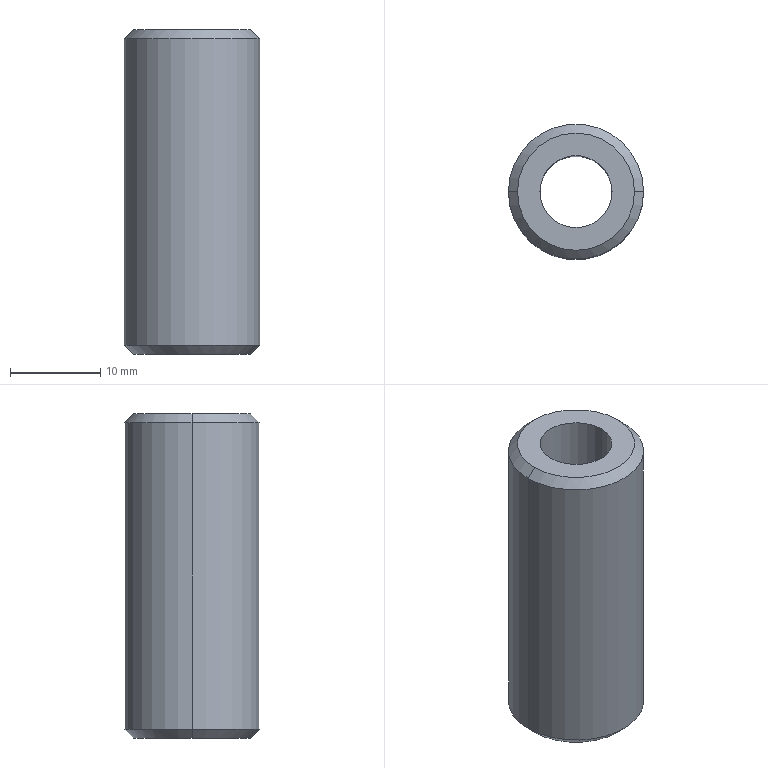Part | SolidWorks | features Chamfer 1, Extrusion 1, ICE 1 | 1 solid | 10 faces | box 15 x 15 x 36 mm | volume 4507 mm3 | cylinder 4 | cone 4 | plane 2 | commonest cylinder face diameters 8 x2 15 x2
STEP:
#1=CARTESIAN_POINT('',(-4.,0.,0.));
#2=VERTEX_POINT('',#1);
#3=CARTESIAN_POINT('',(4.,0.,0.));
#4=VERTEX_POINT('',#3);
#5=CARTESIAN_POINT('',(0.,0.,0.));
#6=DIRECTION('',(0.,0.,1.));
#7=DIRECTION('',(1.,0.,0.));
#8=AXIS2_PLACEMENT_3D('',#5,#6,#7);
#9=CIRCLE('',#8,4.);
#10=EDGE_CURVE('',#2,#4,#9,.T.);
#11=ORIENTED_EDGE('',*,*,#10,.F.);
#12=CARTESIAN_POINT('',(-4.,0.,36.));
#13=VERTEX_POINT('',#12);
#14=CARTESIAN_POINT('',(-4.,0.,0.));
#15=DIRECTION('',(0.,0.,1.));
#16=VECTOR('',#15,1000.);
#17=LINE('',#14,#16);
#18=EDGE_CURVE('',#2,#13,#17,.T.);
#19=ORIENTED_EDGE('',*,*,#18,.T.);
#20=CARTESIAN_POINT('',(4.,0.,36.));
#21=VERTEX_POINT('',#20);
#22=CARTESIAN_POINT('',(0.,0.,36.));
#23=DIRECTION('',(0.,0.,1.));
#24=DIRECTION('',(1.,0.,0.));
#25=AXIS2_PLACEMENT_3D('',#22,#23,#24);
#26=CIRCLE('',#25,4.);
#27=EDGE_CURVE('',#13,#21,#26,.T.);
#28=ORIENTED_EDGE('',*,*,#27,.T.);
#29=CARTESIAN_POINT('',(4.,0.,0.));
#30=DIRECTION('',(0.,0.,1.));
#31=VECTOR('',#30,1000.);
#32=LINE('',#29,#31);
#33=EDGE_CURVE('',#4,#21,#32,.T.);
#34=ORIENTED_EDGE('',*,*,#33,.F.);
#35=EDGE_LOOP('',(#11,#19,#28,#34));
#36=FACE_OUTER_BOUND('',#35,.T.);
#37=CARTESIAN_POINT('',(0.,0.,0.));
#38=DIRECTION('',(0.,0.,1.));
#39=DIRECTION('',(1.,0.,0.));
#40=AXIS2_PLACEMENT_3D('',#37,#38,#39);
#41=CYLINDRICAL_SURFACE('',#40,4.);
#42=ADVANCED_FACE('',(#36),#41,.F.);
#43=CARTESIAN_POINT('',(6.5,0.,36.));
#44=VERTEX_POINT('',#43);
#45=CARTESIAN_POINT('',(-6.5,0.,36.));
#46=VERTEX_POINT('',#45);
#47=CARTESIAN_POINT('',(0.,0.,36.));
#48=DIRECTION('',(0.,0.,1.));
#49=DIRECTION('',(1.,0.,0.));
#50=AXIS2_PLACEMENT_3D('',#47,#48,#49);
#51=CIRCLE('',#50,6.5);
#52=EDGE_CURVE('',#44,#46,#51,.T.);
#53=ORIENTED_EDGE('',*,*,#52,.F.);
#54=CARTESIAN_POINT('',(7.5,0.,35.));
#55=VERTEX_POINT('',#54);
#56=CARTESIAN_POINT('',(6.5,0.,36.));
#57=DIRECTION('',(0.7071,0.,-0.7071));
#58=VECTOR('',#57,1000.);
#59=LINE('',#56,#58);
#60=EDGE_CURVE('',#44,#55,#59,.T.);
#61=ORIENTED_EDGE('',*,*,#60,.T.);
#62=CARTESIAN_POINT('',(-7.5,0.,35.));
#63=VERTEX_POINT('',#62);
#64=CARTESIAN_POINT('',(0.,0.,35.));
#65=DIRECTION('',(0.,0.,-1.));
#66=DIRECTION('',(1.,0.,0.));
#67=AXIS2_PLACEMENT_3D('',#64,#65,#66);
#68=CIRCLE('',#67,7.5);
#69=EDGE_CURVE('',#63,#55,#68,.T.);
#70=ORIENTED_EDGE('',*,*,#69,.F.);
#71=CARTESIAN_POINT('',(-6.5,0.,36.));
#72=DIRECTION('',(-0.7071,0.,-0.7071));
#73=VECTOR('',#72,1000.);
#74=LINE('',#71,#73);
#75=EDGE_CURVE('',#46,#63,#74,.T.);
#76=ORIENTED_EDGE('',*,*,#75,.F.);
#77=EDGE_LOOP('',(#53,#61,#70,#76));
#78=FACE_OUTER_BOUND('',#77,.T.);
#79=CARTESIAN_POINT('',(0.,0.,36.));
#80=DIRECTION('',(0.,0.,-1.));
#81=DIRECTION('',(-1.,0.,0.));
#82=AXIS2_PLACEMENT_3D('',#79,#80,#81);
#83=CONICAL_SURFACE('',#82,6.5,0.7854);
#84=ADVANCED_FACE('',(#78),#83,.T.);
#85=CARTESIAN_POINT('',(-6.5,0.,0.));
#86=VERTEX_POINT('',#85);
#87=CARTESIAN_POINT('',(6.5,0.,0.));
#88=VERTEX_POINT('',#87);
#89=CARTESIAN_POINT('',(0.,0.,0.));
#90=DIRECTION('',(0.,0.,-1.));
#91=DIRECTION('',(1.,0.,0.));
#92=AXIS2_PLACEMENT_3D('',#89,#90,#91);
#93=CIRCLE('',#92,6.5);
#94=EDGE_CURVE('',#86,#88,#93,.T.);
#95=ORIENTED_EDGE('',*,*,#94,.F.);
#96=CARTESIAN_POINT('',(-7.5,0.,1.));
#97=VERTEX_POINT('',#96);
#98=CARTESIAN_POINT('',(-7.5,0.,1.));
#99=DIRECTION('',(-0.7071,0.,0.7071));
#100=VECTOR('',#99,1000.);
#101=LINE('',#98,#100);
#102=EDGE_CURVE('',#86,#97,#101,.T.);
#103=ORIENTED_EDGE('',*,*,#102,.T.);
#104=CARTESIAN_POINT('',(7.5,0.,1.));
#105=VERTEX_POINT('',#104);
#106=CARTESIAN_POINT('',(0.,0.,1.));
#107=DIRECTION('',(0.,0.,1.));
#108=DIRECTION('',(1.,0.,0.));
#109=AXIS2_PLACEMENT_3D('',#106,#107,#108);
#110=CIRCLE('',#109,7.5);
#111=EDGE_CURVE('',#105,#97,#110,.T.);
#112=ORIENTED_EDGE('',*,*,#111,.F.);
#113=CARTESIAN_POINT('',(7.5,0.,1.));
#114=DIRECTION('',(0.7071,0.,0.7071));
#115=VECTOR('',#114,1000.);
#116=LINE('',#113,#115);
#117=EDGE_CURVE('',#88,#105,#116,.T.);
#118=ORIENTED_EDGE('',*,*,#117,.F.);
#119=EDGE_LOOP('',(#95,#103,#112,#118));
#120=FACE_OUTER_BOUND('',#119,.T.);
#121=CARTESIAN_POINT('',(0.,0.,1.));
#122=DIRECTION('',(0.,0.,1.));
#123=DIRECTION('',(1.,0.,0.));
#124=AXIS2_PLACEMENT_3D('',#121,#122,#123);
#125=CONICAL_SURFACE('',#124,7.5,0.7854);
#126=ADVANCED_FACE('',(#120),#125,.T.);
#127=ORIENTED_EDGE('',*,*,#69,.T.);
#128=CARTESIAN_POINT('',(7.5,0.,36.));
#129=DIRECTION('',(0.,0.,-1.));
#130=VECTOR('',#129,1000.);
#131=LINE('',#128,#130);
#132=EDGE_CURVE('',#55,#105,#131,.T.);
#133=ORIENTED_EDGE('',*,*,#132,.T.);
#134=ORIENTED_EDGE('',*,*,#111,.T.);
#135=CARTESIAN_POINT('',(-7.5,0.,36.));
#136=DIRECTION('',(0.,0.,-1.));
#137=VECTOR('',#136,1000.);
#138=LINE('',#135,#137);
#139=EDGE_CURVE('',#63,#97,#138,.T.);
#140=ORIENTED_EDGE('',*,*,#139,.F.);
#141=EDGE_LOOP('',(#127,#133,#134,#140));
#142=FACE_OUTER_BOUND('',#141,.T.);
#143=CARTESIAN_POINT('',(0.,0.,36.));
#144=DIRECTION('',(0.,0.,-1.));
#145=DIRECTION('',(-1.,0.,0.));
#146=AXIS2_PLACEMENT_3D('',#143,#144,#145);
#147=CYLINDRICAL_SURFACE('',#146,7.5);
#148=ADVANCED_FACE('',(#142),#147,.T.);
#149=ORIENTED_EDGE('',*,*,#132,.F.);
#150=CARTESIAN_POINT('',(0.,0.,35.));
#151=DIRECTION('',(0.,0.,-1.));
#152=DIRECTION('',(1.,0.,0.));
#153=AXIS2_PLACEMENT_3D('',#150,#151,#152);
#154=CIRCLE('',#153,7.5);
#155=EDGE_CURVE('',#55,#63,#154,.T.);
#156=ORIENTED_EDGE('',*,*,#155,.T.);
#157=ORIENTED_EDGE('',*,*,#139,.T.);
#158=CARTESIAN_POINT('',(0.,0.,1.));
#159=DIRECTION('',(0.,0.,1.));
#160=DIRECTION('',(1.,0.,0.));
#161=AXIS2_PLACEMENT_3D('',#158,#159,#160);
#162=CIRCLE('',#161,7.5);
#163=EDGE_CURVE('',#97,#105,#162,.T.);
#164=ORIENTED_EDGE('',*,*,#163,.T.);
#165=EDGE_LOOP('',(#149,#156,#157,#164));
#166=FACE_OUTER_BOUND('',#165,.T.);
#167=CARTESIAN_POINT('',(0.,0.,36.));
#168=DIRECTION('',(0.,0.,-1.));
#169=DIRECTION('',(-1.,0.,0.));
#170=AXIS2_PLACEMENT_3D('',#167,#168,#169);
#171=CYLINDRICAL_SURFACE('',#170,7.5);
#172=ADVANCED_FACE('',(#166),#171,.T.);
#173=CARTESIAN_POINT('',(0.,0.,36.));
#174=DIRECTION('',(0.,0.,1.));
#175=DIRECTION('',(1.,0.,0.));
#176=AXIS2_PLACEMENT_3D('',#173,#174,#175);
#177=CIRCLE('',#176,4.);
#178=EDGE_CURVE('',#21,#13,#177,.T.);
#179=ORIENTED_EDGE('',*,*,#178,.F.);
#180=ORIENTED_EDGE('',*,*,#27,.F.);
#181=EDGE_LOOP('',(#179,#180));
#182=FACE_BOUND('',#181,.T.);
#183=CARTESIAN_POINT('',(0.,0.,36.));
#184=DIRECTION('',(0.,0.,1.));
#185=DIRECTION('',(1.,0.,0.));
#186=AXIS2_PLACEMENT_3D('',#183,#184,#185);
#187=CIRCLE('',#186,6.5);
#188=EDGE_CURVE('',#46,#44,#187,.T.);
#189=ORIENTED_EDGE('',*,*,#188,.T.);
#190=ORIENTED_EDGE('',*,*,#52,.T.);
#191=EDGE_LOOP('',(#189,#190));
#192=FACE_OUTER_BOUND('',#191,.T.);
#193=CARTESIAN_POINT('',(0.,0.,36.));
#194=DIRECTION('',(0.,0.,1.));
#195=DIRECTION('',(1.,0.,0.));
#196=AXIS2_PLACEMENT_3D('',#193,#194,#195);
#197=PLANE('',#196);
#198=ADVANCED_FACE('',(#182,#192),#197,.T.);
#199=CARTESIAN_POINT('',(0.,0.,0.));
#200=DIRECTION('',(0.,0.,1.));
#201=DIRECTION('',(1.,0.,0.));
#202=AXIS2_PLACEMENT_3D('',#199,#200,#201);
#203=CIRCLE('',#202,4.);
#204=EDGE_CURVE('',#4,#2,#203,.T.);
#205=ORIENTED_EDGE('',*,*,#204,.T.);
#206=ORIENTED_EDGE('',*,*,#10,.T.);
#207=EDGE_LOOP('',(#205,#206));
#208=FACE_BOUND('',#207,.T.);
#209=CARTESIAN_POINT('',(0.,0.,0.));
#210=DIRECTION('',(0.,0.,-1.));
#211=DIRECTION('',(1.,0.,0.));
#212=AXIS2_PLACEMENT_3D('',#209,#210,#211);
#213=CIRCLE('',#212,6.5);
#214=EDGE_CURVE('',#88,#86,#213,.T.);
#215=ORIENTED_EDGE('',*,*,#214,.T.);
#216=ORIENTED_EDGE('',*,*,#94,.T.);
#217=EDGE_LOOP('',(#215,#216));
#218=FACE_OUTER_BOUND('',#217,.T.);
#219=CARTESIAN_POINT('',(0.,0.,0.));
#220=DIRECTION('',(0.,0.,1.));
#221=DIRECTION('',(1.,0.,0.));
#222=AXIS2_PLACEMENT_3D('',#219,#220,#221);
#223=PLANE('',#222);
#224=ADVANCED_FACE('',(#208,#218),#223,.F.);
#225=ORIENTED_EDGE('',*,*,#102,.F.);
#226=ORIENTED_EDGE('',*,*,#214,.F.);
#227=ORIENTED_EDGE('',*,*,#117,.T.);
#228=ORIENTED_EDGE('',*,*,#163,.F.);
#229=EDGE_LOOP('',(#225,#226,#227,#228));
#230=FACE_OUTER_BOUND('',#229,.T.);
#231=CARTESIAN_POINT('',(0.,0.,1.));
#232=DIRECTION('',(0.,0.,1.));
#233=DIRECTION('',(1.,0.,0.));
#234=AXIS2_PLACEMENT_3D('',#231,#232,#233);
#235=CONICAL_SURFACE('',#234,7.5,0.7854);
#236=ADVANCED_FACE('',(#230),#235,.T.);
#237=ORIENTED_EDGE('',*,*,#60,.F.);
#238=ORIENTED_EDGE('',*,*,#188,.F.);
#239=ORIENTED_EDGE('',*,*,#75,.T.);
#240=ORIENTED_EDGE('',*,*,#155,.F.);
#241=EDGE_LOOP('',(#237,#238,#239,#240));
#242=FACE_OUTER_BOUND('',#241,.T.);
#243=CARTESIAN_POINT('',(0.,0.,36.));
#244=DIRECTION('',(0.,0.,-1.));
#245=DIRECTION('',(-1.,0.,0.));
#246=AXIS2_PLACEMENT_3D('',#243,#244,#245);
#247=CONICAL_SURFACE('',#246,6.5,0.7854);
#248=ADVANCED_FACE('',(#242),#247,.T.);
#249=ORIENTED_EDGE('',*,*,#18,.F.);
#250=ORIENTED_EDGE('',*,*,#204,.F.);
#251=ORIENTED_EDGE('',*,*,#33,.T.);
#252=ORIENTED_EDGE('',*,*,#178,.T.);
#253=EDGE_LOOP('',(#249,#250,#251,#252));
#254=FACE_OUTER_BOUND('',#253,.T.);
#255=CARTESIAN_POINT('',(0.,0.,0.));
#256=DIRECTION('',(0.,0.,1.));
#257=DIRECTION('',(1.,0.,0.));
#258=AXIS2_PLACEMENT_3D('',#255,#256,#257);
#259=CYLINDRICAL_SURFACE('',#258,4.);
#260=ADVANCED_FACE('',(#254),#259,.F.);
#261=CLOSED_SHELL('',(#42,#84,#126,#148,#172,#198,#224,#236,#248,#260));
#262=MANIFOLD_SOLID_BREP('',#261);
#263=CARTESIAN_POINT('',(0.,0.,0.));
#264=DIRECTION('',(0.,0.,1.));
#265=DIRECTION('',(1.,0.,0.));
#266=AXIS2_PLACEMENT_3D('',#263,#264,#265);
#267=(LENGTH_UNIT()NAMED_UNIT(*)SI_UNIT(.MILLI.,.METRE.));
#268=UNCERTAINTY_MEASURE_WITH_UNIT(LENGTH_MEASURE(0.00001),#267,'','');
#269=(NAMED_UNIT(*)PLANE_ANGLE_UNIT()SI_UNIT($,.RADIAN.));
#270=(NAMED_UNIT(*)SI_UNIT($,.STERADIAN.)SOLID_ANGLE_UNIT());
#271=(GEOMETRIC_REPRESENTATION_CONTEXT(3)GLOBAL_UNCERTAINTY_ASSIGNED_CONTEXT((#268))GLOBAL_UNIT_ASSIGNED_CONTEXT((#267,#269,#270))REPRESENTATION_CONTEXT('',''));
#272=ADVANCED_BREP_SHAPE_REPRESENTATION('',(#262,#266),#271);